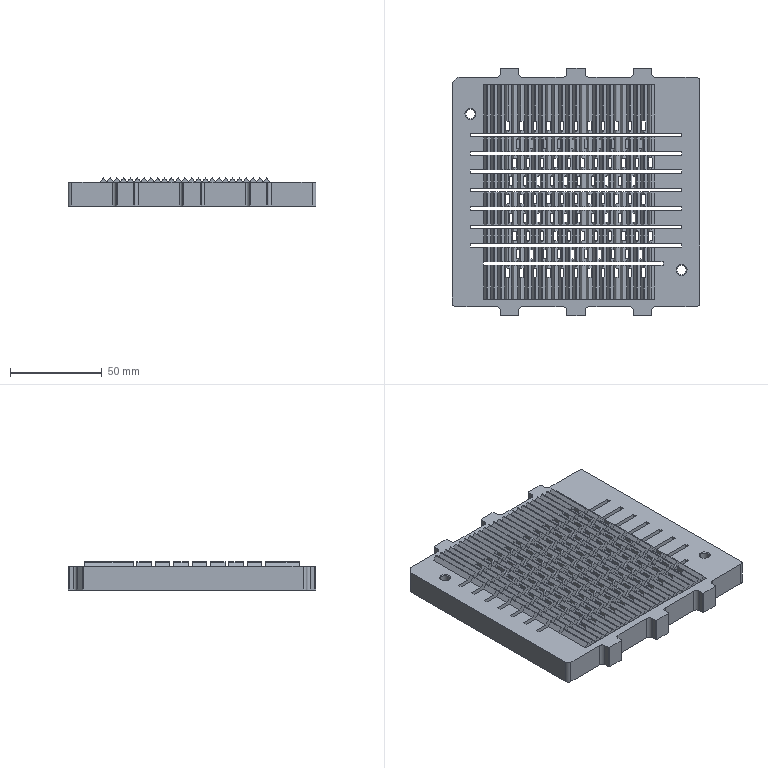Part | STEP file | 200 mesh_id2070 | 1 solid | 1466 faces | box 135 x 135 x 15.259 mm | volume 197711 mm3 | plane 895 | cylinder 567 | cone 4 | commonest cylinder face diameters 0.5 x536 4 x15 1 x14 5 x2